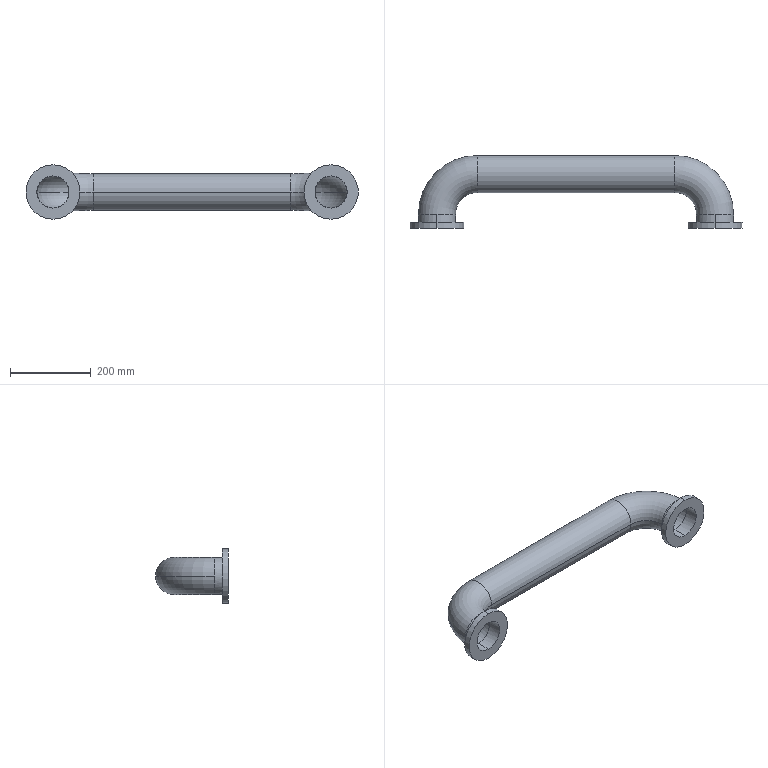Part | SolidWorks | features ICE 1, Sweep 1 | 1 solid | 28 faces | box 825 x 181 x 135 mm | volume 1647054 mm3 | cylinder 16 | torus 8 | plane 4 | commonest cylinder face diameters 80 x6 92 x6 135 x4
STEP:
#1=CARTESIAN_POINT('',(590.,80.,0.));
#2=VERTEX_POINT('',#1);
#3=CARTESIAN_POINT('',(590.,160.,0.));
#4=VERTEX_POINT('',#3);
#5=CARTESIAN_POINT('',(590.,120.,0.));
#6=DIRECTION('',(-1.,0.,0.));
#7=DIRECTION('',(0.,0.,1.));
#8=AXIS2_PLACEMENT_3D('',#5,#6,#7);
#9=CIRCLE('',#8,40.);
#10=EDGE_CURVE('',#2,#4,#9,.T.);
#11=ORIENTED_EDGE('',*,*,#10,.T.);
#12=CARTESIAN_POINT('',(730.,20.,0.));
#13=VERTEX_POINT('',#12);
#14=CARTESIAN_POINT('',(590.,20.,0.));
#15=DIRECTION('',(0.,0.,-1.));
#16=DIRECTION('',(-1.,0.,0.));
#17=AXIS2_PLACEMENT_3D('',#14,#15,#16);
#18=CIRCLE('',#17,140.);
#19=EDGE_CURVE('',#4,#13,#18,.T.);
#20=ORIENTED_EDGE('',*,*,#19,.T.);
#21=CARTESIAN_POINT('',(690.,20.,40.));
#22=VERTEX_POINT('',#21);
#23=CARTESIAN_POINT('',(690.,20.,0.));
#24=DIRECTION('',(0.,1.,0.));
#25=DIRECTION('',(0.,0.,1.));
#26=AXIS2_PLACEMENT_3D('',#23,#24,#25);
#27=CIRCLE('',#26,40.);
#28=EDGE_CURVE('',#22,#13,#27,.T.);
#29=ORIENTED_EDGE('',*,*,#28,.F.);
#30=CARTESIAN_POINT('',(650.,20.,0.));
#31=VERTEX_POINT('',#30);
#32=CARTESIAN_POINT('',(690.,20.,0.));
#33=DIRECTION('',(0.,1.,0.));
#34=DIRECTION('',(0.,0.,1.));
#35=AXIS2_PLACEMENT_3D('',#32,#33,#34);
#36=CIRCLE('',#35,40.);
#37=EDGE_CURVE('',#31,#22,#36,.T.);
#38=ORIENTED_EDGE('',*,*,#37,.F.);
#39=CARTESIAN_POINT('',(590.,20.,0.));
#40=DIRECTION('',(0.,0.,-1.));
#41=DIRECTION('',(-1.,0.,0.));
#42=AXIS2_PLACEMENT_3D('',#39,#40,#41);
#43=CIRCLE('',#42,60.);
#44=EDGE_CURVE('',#2,#31,#43,.T.);
#45=ORIENTED_EDGE('',*,*,#44,.F.);
#46=EDGE_LOOP('',(#11,#20,#29,#38,#45));
#47=FACE_OUTER_BOUND('',#46,.T.);
#48=CARTESIAN_POINT('',(590.,20.,0.));
#49=DIRECTION('',(0.,0.,-1.));
#50=DIRECTION('',(-1.,0.,0.));
#51=AXIS2_PLACEMENT_3D('',#48,#49,#50);
#52=TOROIDAL_SURFACE('',#51,100.,40.);
#53=ADVANCED_FACE('',(#47),#52,.F.);
#54=CARTESIAN_POINT('',(0.,20.,40.));
#55=VERTEX_POINT('',#54);
#56=CARTESIAN_POINT('',(-40.,20.,0.));
#57=VERTEX_POINT('',#56);
#58=CARTESIAN_POINT('',(0.,20.,0.));
#59=DIRECTION('',(0.,-1.,0.));
#60=DIRECTION('',(0.,0.,1.));
#61=AXIS2_PLACEMENT_3D('',#58,#59,#60);
#62=CIRCLE('',#61,40.);
#63=EDGE_CURVE('',#55,#57,#62,.T.);
#64=ORIENTED_EDGE('',*,*,#63,.T.);
#65=CARTESIAN_POINT('',(100.,160.,0.));
#66=VERTEX_POINT('',#65);
#67=CARTESIAN_POINT('',(100.,20.,0.));
#68=DIRECTION('',(0.,0.,-1.));
#69=DIRECTION('',(-1.,0.,0.));
#70=AXIS2_PLACEMENT_3D('',#67,#68,#69);
#71=CIRCLE('',#70,140.);
#72=EDGE_CURVE('',#57,#66,#71,.T.);
#73=ORIENTED_EDGE('',*,*,#72,.T.);
#74=CARTESIAN_POINT('',(100.,80.,0.));
#75=VERTEX_POINT('',#74);
#76=CARTESIAN_POINT('',(100.,120.,0.));
#77=DIRECTION('',(-1.,0.,0.));
#78=DIRECTION('',(0.,0.,1.));
#79=AXIS2_PLACEMENT_3D('',#76,#77,#78);
#80=CIRCLE('',#79,40.);
#81=EDGE_CURVE('',#75,#66,#80,.T.);
#82=ORIENTED_EDGE('',*,*,#81,.F.);
#83=CARTESIAN_POINT('',(40.,20.,0.));
#84=VERTEX_POINT('',#83);
#85=CARTESIAN_POINT('',(100.,20.,0.));
#86=DIRECTION('',(0.,0.,-1.));
#87=DIRECTION('',(-1.,0.,0.));
#88=AXIS2_PLACEMENT_3D('',#85,#86,#87);
#89=CIRCLE('',#88,60.);
#90=EDGE_CURVE('',#84,#75,#89,.T.);
#91=ORIENTED_EDGE('',*,*,#90,.F.);
#92=CARTESIAN_POINT('',(0.,20.,0.));
#93=DIRECTION('',(0.,-1.,0.));
#94=DIRECTION('',(0.,0.,1.));
#95=AXIS2_PLACEMENT_3D('',#92,#93,#94);
#96=CIRCLE('',#95,40.);
#97=EDGE_CURVE('',#84,#55,#96,.T.);
#98=ORIENTED_EDGE('',*,*,#97,.T.);
#99=EDGE_LOOP('',(#64,#73,#82,#91,#98));
#100=FACE_OUTER_BOUND('',#99,.T.);
#101=CARTESIAN_POINT('',(100.,20.,0.));
#102=DIRECTION('',(0.,0.,-1.));
#103=DIRECTION('',(-1.,0.,0.));
#104=AXIS2_PLACEMENT_3D('',#101,#102,#103);
#105=TOROIDAL_SURFACE('',#104,100.,40.);
#106=ADVANCED_FACE('',(#100),#105,.F.);
#107=CARTESIAN_POINT('',(590.,74.,0.));
#108=VERTEX_POINT('',#107);
#109=CARTESIAN_POINT('',(590.,166.,0.));
#110=VERTEX_POINT('',#109);
#111=CARTESIAN_POINT('',(590.,120.,0.));
#112=DIRECTION('',(1.,0.,0.));
#113=DIRECTION('',(0.,0.,1.));
#114=AXIS2_PLACEMENT_3D('',#111,#112,#113);
#115=CIRCLE('',#114,46.);
#116=EDGE_CURVE('',#108,#110,#115,.T.);
#117=ORIENTED_EDGE('',*,*,#116,.T.);
#118=CARTESIAN_POINT('',(736.,20.,0.));
#119=VERTEX_POINT('',#118);
#120=CARTESIAN_POINT('',(590.,20.,0.));
#121=DIRECTION('',(0.,0.,-1.));
#122=DIRECTION('',(-1.,0.,0.));
#123=AXIS2_PLACEMENT_3D('',#120,#121,#122);
#124=CIRCLE('',#123,146.);
#125=EDGE_CURVE('',#110,#119,#124,.T.);
#126=ORIENTED_EDGE('',*,*,#125,.T.);
#127=CARTESIAN_POINT('',(690.,20.,-46.));
#128=VERTEX_POINT('',#127);
#129=CARTESIAN_POINT('',(690.,20.,0.));
#130=DIRECTION('',(0.,-1.,0.));
#131=DIRECTION('',(0.,0.,1.));
#132=AXIS2_PLACEMENT_3D('',#129,#130,#131);
#133=CIRCLE('',#132,46.);
#134=EDGE_CURVE('',#128,#119,#133,.T.);
#135=ORIENTED_EDGE('',*,*,#134,.F.);
#136=CARTESIAN_POINT('',(644.,20.,0.));
#137=VERTEX_POINT('',#136);
#138=CARTESIAN_POINT('',(690.,20.,0.));
#139=DIRECTION('',(0.,-1.,0.));
#140=DIRECTION('',(0.,0.,1.));
#141=AXIS2_PLACEMENT_3D('',#138,#139,#140);
#142=CIRCLE('',#141,46.);
#143=EDGE_CURVE('',#137,#128,#142,.T.);
#144=ORIENTED_EDGE('',*,*,#143,.F.);
#145=CARTESIAN_POINT('',(590.,20.,0.));
#146=DIRECTION('',(0.,0.,-1.));
#147=DIRECTION('',(-1.,0.,0.));
#148=AXIS2_PLACEMENT_3D('',#145,#146,#147);
#149=CIRCLE('',#148,54.);
#150=EDGE_CURVE('',#108,#137,#149,.T.);
#151=ORIENTED_EDGE('',*,*,#150,.F.);
#152=EDGE_LOOP('',(#117,#126,#135,#144,#151));
#153=FACE_OUTER_BOUND('',#152,.T.);
#154=CARTESIAN_POINT('',(590.,20.,0.));
#155=DIRECTION('',(0.,0.,-1.));
#156=DIRECTION('',(-1.,0.,0.));
#157=AXIS2_PLACEMENT_3D('',#154,#155,#156);
#158=TOROIDAL_SURFACE('',#157,100.,46.);
#159=ADVANCED_FACE('',(#153),#158,.T.);
#160=CARTESIAN_POINT('',(0.,20.,-46.));
#161=VERTEX_POINT('',#160);
#162=CARTESIAN_POINT('',(-46.,20.,0.));
#163=VERTEX_POINT('',#162);
#164=CARTESIAN_POINT('',(0.,20.,0.));
#165=DIRECTION('',(0.,1.,0.));
#166=DIRECTION('',(0.,0.,1.));
#167=AXIS2_PLACEMENT_3D('',#164,#165,#166);
#168=CIRCLE('',#167,46.);
#169=EDGE_CURVE('',#161,#163,#168,.T.);
#170=ORIENTED_EDGE('',*,*,#169,.T.);
#171=CARTESIAN_POINT('',(100.,166.,0.));
#172=VERTEX_POINT('',#171);
#173=CARTESIAN_POINT('',(100.,20.,0.));
#174=DIRECTION('',(0.,0.,-1.));
#175=DIRECTION('',(-1.,0.,0.));
#176=AXIS2_PLACEMENT_3D('',#173,#174,#175);
#177=CIRCLE('',#176,146.);
#178=EDGE_CURVE('',#163,#172,#177,.T.);
#179=ORIENTED_EDGE('',*,*,#178,.T.);
#180=CARTESIAN_POINT('',(100.,74.,0.));
#181=VERTEX_POINT('',#180);
#182=CARTESIAN_POINT('',(100.,120.,0.));
#183=DIRECTION('',(1.,0.,0.));
#184=DIRECTION('',(0.,0.,1.));
#185=AXIS2_PLACEMENT_3D('',#182,#183,#184);
#186=CIRCLE('',#185,46.);
#187=EDGE_CURVE('',#181,#172,#186,.T.);
#188=ORIENTED_EDGE('',*,*,#187,.F.);
#189=CARTESIAN_POINT('',(46.,20.,0.));
#190=VERTEX_POINT('',#189);
#191=CARTESIAN_POINT('',(100.,20.,0.));
#192=DIRECTION('',(0.,0.,-1.));
#193=DIRECTION('',(-1.,0.,0.));
#194=AXIS2_PLACEMENT_3D('',#191,#192,#193);
#195=CIRCLE('',#194,54.);
#196=EDGE_CURVE('',#190,#181,#195,.T.);
#197=ORIENTED_EDGE('',*,*,#196,.F.);
#198=CARTESIAN_POINT('',(0.,20.,0.));
#199=DIRECTION('',(0.,1.,0.));
#200=DIRECTION('',(0.,0.,1.));
#201=AXIS2_PLACEMENT_3D('',#198,#199,#200);
#202=CIRCLE('',#201,46.);
#203=EDGE_CURVE('',#190,#161,#202,.T.);
#204=ORIENTED_EDGE('',*,*,#203,.T.);
#205=EDGE_LOOP('',(#170,#179,#188,#197,#204));
#206=FACE_OUTER_BOUND('',#205,.T.);
#207=CARTESIAN_POINT('',(100.,20.,0.));
#208=DIRECTION('',(0.,0.,-1.));
#209=DIRECTION('',(-1.,0.,0.));
#210=AXIS2_PLACEMENT_3D('',#207,#208,#209);
#211=TOROIDAL_SURFACE('',#210,100.,46.);
#212=ADVANCED_FACE('',(#206),#211,.T.);
#213=CARTESIAN_POINT('',(690.,-15.,-67.5));
#214=VERTEX_POINT('',#213);
#215=CARTESIAN_POINT('',(690.,-15.,67.5));
#216=VERTEX_POINT('',#215);
#217=CARTESIAN_POINT('',(690.,-15.,0.));
#218=DIRECTION('',(0.,-1.,0.));
#219=DIRECTION('',(0.,0.,-1.));
#220=AXIS2_PLACEMENT_3D('',#217,#218,#219);
#221=CIRCLE('',#220,67.5);
#222=EDGE_CURVE('',#214,#216,#221,.T.);
#223=ORIENTED_EDGE('',*,*,#222,.F.);
#224=CARTESIAN_POINT('',(690.,0.,-67.5));
#225=VERTEX_POINT('',#224);
#226=CARTESIAN_POINT('',(690.,-15.,-67.5));
#227=DIRECTION('',(0.,1.,0.));
#228=VECTOR('',#227,1000.);
#229=LINE('',#226,#228);
#230=EDGE_CURVE('',#214,#225,#229,.T.);
#231=ORIENTED_EDGE('',*,*,#230,.T.);
#232=CARTESIAN_POINT('',(690.,0.,67.5));
#233=VERTEX_POINT('',#232);
#234=CARTESIAN_POINT('',(690.,0.,0.));
#235=DIRECTION('',(0.,-1.,0.));
#236=DIRECTION('',(0.,0.,-1.));
#237=AXIS2_PLACEMENT_3D('',#234,#235,#236);
#238=CIRCLE('',#237,67.5);
#239=EDGE_CURVE('',#225,#233,#238,.T.);
#240=ORIENTED_EDGE('',*,*,#239,.T.);
#241=CARTESIAN_POINT('',(690.,-15.,67.5));
#242=DIRECTION('',(0.,1.,0.));
#243=VECTOR('',#242,1000.);
#244=LINE('',#241,#243);
#245=EDGE_CURVE('',#216,#233,#244,.T.);
#246=ORIENTED_EDGE('',*,*,#245,.F.);
#247=EDGE_LOOP('',(#223,#231,#240,#246));
#248=FACE_OUTER_BOUND('',#247,.T.);
#249=CARTESIAN_POINT('',(690.,-15.,0.));
#250=DIRECTION('',(0.,1.,0.));
#251=DIRECTION('',(0.,0.,1.));
#252=AXIS2_PLACEMENT_3D('',#249,#250,#251);
#253=CYLINDRICAL_SURFACE('',#252,67.5);
#254=ADVANCED_FACE('',(#248),#253,.T.);
#255=CARTESIAN_POINT('',(0.,-15.,-67.5));
#256=VERTEX_POINT('',#255);
#257=CARTESIAN_POINT('',(0.,-15.,67.5));
#258=VERTEX_POINT('',#257);
#259=CARTESIAN_POINT('',(0.,-15.,0.));
#260=DIRECTION('',(0.,-1.,0.));
#261=DIRECTION('',(0.,0.,-1.));
#262=AXIS2_PLACEMENT_3D('',#259,#260,#261);
#263=CIRCLE('',#262,67.5);
#264=EDGE_CURVE('',#256,#258,#263,.T.);
#265=ORIENTED_EDGE('',*,*,#264,.F.);
#266=CARTESIAN_POINT('',(0.,0.,-67.5));
#267=VERTEX_POINT('',#266);
#268=CARTESIAN_POINT('',(0.,-15.,-67.5));
#269=DIRECTION('',(0.,1.,0.));
#270=VECTOR('',#269,1000.);
#271=LINE('',#268,#270);
#272=EDGE_CURVE('',#256,#267,#271,.T.);
#273=ORIENTED_EDGE('',*,*,#272,.T.);
#274=CARTESIAN_POINT('',(0.,0.,67.5));
#275=VERTEX_POINT('',#274);
#276=CARTESIAN_POINT('',(0.,0.,0.));
#277=DIRECTION('',(0.,-1.,0.));
#278=DIRECTION('',(0.,0.,-1.));
#279=AXIS2_PLACEMENT_3D('',#276,#277,#278);
#280=CIRCLE('',#279,67.5);
#281=EDGE_CURVE('',#267,#275,#280,.T.);
#282=ORIENTED_EDGE('',*,*,#281,.T.);
#283=CARTESIAN_POINT('',(0.,-15.,67.5));
#284=DIRECTION('',(0.,1.,0.));
#285=VECTOR('',#284,1000.);
#286=LINE('',#283,#285);
#287=EDGE_CURVE('',#258,#275,#286,.T.);
#288=ORIENTED_EDGE('',*,*,#287,.F.);
#289=EDGE_LOOP('',(#265,#273,#282,#288));
#290=FACE_OUTER_BOUND('',#289,.T.);
#291=CARTESIAN_POINT('',(0.,-15.,0.));
#292=DIRECTION('',(0.,1.,0.));
#293=DIRECTION('',(0.,0.,1.));
#294=AXIS2_PLACEMENT_3D('',#291,#292,#293);
#295=CYLINDRICAL_SURFACE('',#294,67.5);
#296=ADVANCED_FACE('',(#290),#295,.T.);
#297=CARTESIAN_POINT('',(690.,20.,-40.));
#298=VERTEX_POINT('',#297);
#299=CARTESIAN_POINT('',(690.,20.,0.));
#300=DIRECTION('',(0.,1.,0.));
#301=DIRECTION('',(0.,0.,1.));
#302=AXIS2_PLACEMENT_3D('',#299,#300,#301);
#303=CIRCLE('',#302,40.);
#304=EDGE_CURVE('',#298,#31,#303,.T.);
#305=ORIENTED_EDGE('',*,*,#304,.T.);
#306=ORIENTED_EDGE('',*,*,#37,.T.);
#307=CARTESIAN_POINT('',(690.,-15.,40.));
#308=VERTEX_POINT('',#307);
#309=CARTESIAN_POINT('',(690.,20.,40.));
#310=DIRECTION('',(0.,-1.,0.));
#311=VECTOR('',#310,1000.);
#312=LINE('',#309,#311);
#313=EDGE_CURVE('',#22,#308,#312,.T.);
#314=ORIENTED_EDGE('',*,*,#313,.T.);
#315=CARTESIAN_POINT('',(690.,-15.,-40.));
#316=VERTEX_POINT('',#315);
#317=CARTESIAN_POINT('',(690.,-15.,0.));
#318=DIRECTION('',(0.,-1.,0.));
#319=DIRECTION('',(0.,0.,-1.));
#320=AXIS2_PLACEMENT_3D('',#317,#318,#319);
#321=CIRCLE('',#320,40.);
#322=EDGE_CURVE('',#308,#316,#321,.T.);
#323=ORIENTED_EDGE('',*,*,#322,.T.);
#324=CARTESIAN_POINT('',(690.,20.,-40.));
#325=DIRECTION('',(0.,-1.,0.));
#326=VECTOR('',#325,1000.);
#327=LINE('',#324,#326);
#328=EDGE_CURVE('',#298,#316,#327,.T.);
#329=ORIENTED_EDGE('',*,*,#328,.F.);
#330=EDGE_LOOP('',(#305,#306,#314,#323,#329));
#331=FACE_OUTER_BOUND('',#330,.T.);
#332=CARTESIAN_POINT('',(690.,20.,0.));
#333=DIRECTION('',(0.,-1.,0.));
#334=DIRECTION('',(0.,0.,-1.));
#335=AXIS2_PLACEMENT_3D('',#332,#333,#334);
#336=CYLINDRICAL_SURFACE('',#335,40.);
#337=ADVANCED_FACE('',(#331),#336,.F.);
#338=CARTESIAN_POINT('',(100.,120.,0.));
#339=DIRECTION('',(-1.,0.,0.));
#340=DIRECTION('',(0.,0.,1.));
#341=AXIS2_PLACEMENT_3D('',#338,#339,#340);
#342=CIRCLE('',#341,40.);
#343=EDGE_CURVE('',#66,#75,#342,.T.);
#344=ORIENTED_EDGE('',*,*,#343,.T.);
#345=CARTESIAN_POINT('',(100.,80.,0.));
#346=DIRECTION('',(1.,0.,0.));
#347=VECTOR('',#346,1000.);
#348=LINE('',#345,#347);
#349=EDGE_CURVE('',#75,#2,#348,.T.);
#350=ORIENTED_EDGE('',*,*,#349,.T.);
#351=CARTESIAN_POINT('',(590.,120.,0.));
#352=DIRECTION('',(-1.,0.,0.));
#353=DIRECTION('',(0.,0.,1.));
#354=AXIS2_PLACEMENT_3D('',#351,#352,#353);
#355=CIRCLE('',#354,40.);
#356=EDGE_CURVE('',#4,#2,#355,.T.);
#357=ORIENTED_EDGE('',*,*,#356,.F.);
#358=CARTESIAN_POINT('',(100.,160.,0.));
#359=DIRECTION('',(1.,0.,0.));
#360=VECTOR('',#359,1000.);
#361=LINE('',#358,#360);
#362=EDGE_CURVE('',#66,#4,#361,.T.);
#363=ORIENTED_EDGE('',*,*,#362,.F.);
#364=EDGE_LOOP('',(#344,#350,#357,#363));
#365=FACE_OUTER_BOUND('',#364,.T.);
#366=CARTESIAN_POINT('',(100.,120.,0.));
#367=DIRECTION('',(1.,0.,0.));
#368=DIRECTION('',(0.,1.,0.));
#369=AXIS2_PLACEMENT_3D('',#366,#367,#368);
#370=CYLINDRICAL_SURFACE('',#369,40.);
#371=ADVANCED_FACE('',(#365),#370,.F.);
#372=CARTESIAN_POINT('',(0.,-15.,40.));
#373=VERTEX_POINT('',#372);
#374=CARTESIAN_POINT('',(0.,-15.,-40.));
#375=VERTEX_POINT('',#374);
#376=CARTESIAN_POINT('',(0.,-15.,0.));
#377=DIRECTION('',(0.,-1.,0.));
#378=DIRECTION('',(0.,0.,-1.));
#379=AXIS2_PLACEMENT_3D('',#376,#377,#378);
#380=CIRCLE('',#379,40.);
#381=EDGE_CURVE('',#373,#375,#380,.T.);
#382=ORIENTED_EDGE('',*,*,#381,.T.);
#383=CARTESIAN_POINT('',(0.,20.,-40.));
#384=VERTEX_POINT('',#383);
#385=CARTESIAN_POINT('',(0.,0.,-40.));
#386=DIRECTION('',(0.,1.,0.));
#387=VECTOR('',#386,1000.);
#388=LINE('',#385,#387);
#389=EDGE_CURVE('',#375,#384,#388,.T.);
#390=ORIENTED_EDGE('',*,*,#389,.T.);
#391=CARTESIAN_POINT('',(0.,20.,0.));
#392=DIRECTION('',(0.,-1.,0.));
#393=DIRECTION('',(0.,0.,1.));
#394=AXIS2_PLACEMENT_3D('',#391,#392,#393);
#395=CIRCLE('',#394,40.);
#396=EDGE_CURVE('',#57,#384,#395,.T.);
#397=ORIENTED_EDGE('',*,*,#396,.F.);
#398=ORIENTED_EDGE('',*,*,#63,.F.);
#399=CARTESIAN_POINT('',(0.,0.,40.));
#400=DIRECTION('',(0.,1.,0.));
#401=VECTOR('',#400,1000.);
#402=LINE('',#399,#401);
#403=EDGE_CURVE('',#373,#55,#402,.T.);
#404=ORIENTED_EDGE('',*,*,#403,.F.);
#405=EDGE_LOOP('',(#382,#390,#397,#398,#404));
#406=FACE_OUTER_BOUND('',#405,.T.);
#407=CARTESIAN_POINT('',(0.,0.,0.));
#408=DIRECTION('',(0.,1.,0.));
#409=DIRECTION('',(0.,0.,1.));
#410=AXIS2_PLACEMENT_3D('',#407,#408,#409);
#411=CYLINDRICAL_SURFACE('',#410,40.);
#412=ADVANCED_FACE('',(#406),#411,.F.);
#413=ORIENTED_EDGE('',*,*,#134,.T.);
#414=CARTESIAN_POINT('',(690.,20.,46.));
#415=VERTEX_POINT('',#414);
#416=CARTESIAN_POINT('',(690.,20.,0.));
#417=DIRECTION('',(0.,-1.,0.));
#418=DIRECTION('',(0.,0.,1.));
#419=AXIS2_PLACEMENT_3D('',#416,#417,#418);
#420=CIRCLE('',#419,46.);
#421=EDGE_CURVE('',#119,#415,#420,.T.);
#422=ORIENTED_EDGE('',*,*,#421,.T.);
#423=CARTESIAN_POINT('',(690.,0.,46.));
#424=VERTEX_POINT('',#423);
#425=CARTESIAN_POINT('',(690.,20.,46.));
#426=DIRECTION('',(0.,-1.,0.));
#427=VECTOR('',#426,1000.);
#428=LINE('',#425,#427);
#429=EDGE_CURVE('',#415,#424,#428,.T.);
#430=ORIENTED_EDGE('',*,*,#429,.T.);
#431=CARTESIAN_POINT('',(690.,0.,-46.));
#432=VERTEX_POINT('',#431);
#433=CARTESIAN_POINT('',(690.,0.,0.));
#434=DIRECTION('',(0.,-1.,0.));
#435=DIRECTION('',(0.,0.,1.));
#436=AXIS2_PLACEMENT_3D('',#433,#434,#435);
#437=CIRCLE('',#436,46.);
#438=EDGE_CURVE('',#432,#424,#437,.T.);
#439=ORIENTED_EDGE('',*,*,#438,.F.);
#440=CARTESIAN_POINT('',(690.,20.,-46.));
#441=DIRECTION('',(0.,-1.,0.));
#442=VECTOR('',#441,1000.);
#443=LINE('',#440,#442);
#444=EDGE_CURVE('',#128,#432,#443,.T.);
#445=ORIENTED_EDGE('',*,*,#444,.F.);
#446=EDGE_LOOP('',(#413,#422,#430,#439,#445));
#447=FACE_OUTER_BOUND('',#446,.T.);
#448=CARTESIAN_POINT('',(690.,20.,0.));
#449=DIRECTION('',(0.,-1.,0.));
#450=DIRECTION('',(0.,0.,-1.));
#451=AXIS2_PLACEMENT_3D('',#448,#449,#450);
#452=CYLINDRICAL_SURFACE('',#451,46.);
#453=ADVANCED_FACE('',(#447),#452,.T.);
#454=CARTESIAN_POINT('',(100.,120.,0.));
#455=DIRECTION('',(1.,0.,0.));
#456=DIRECTION('',(0.,0.,1.));
#457=AXIS2_PLACEMENT_3D('',#454,#455,#456);
#458=CIRCLE('',#457,46.);
#459=EDGE_CURVE('',#172,#181,#458,.T.);
#460=ORIENTED_EDGE('',*,*,#459,.T.);
#461=CARTESIAN_POINT('',(100.,74.,0.));
#462=DIRECTION('',(1.,0.,0.));
#463=VECTOR('',#462,1000.);
#464=LINE('',#461,#463);
#465=EDGE_CURVE('',#181,#108,#464,.T.);
#466=ORIENTED_EDGE('',*,*,#465,.T.);
#467=CARTESIAN_POINT('',(590.,120.,0.));
#468=DIRECTION('',(1.,0.,0.));
#469=DIRECTION('',(0.,0.,1.));
#470=AXIS2_PLACEMENT_3D('',#467,#468,#469);
#471=CIRCLE('',#470,46.);
#472=EDGE_CURVE('',#110,#108,#471,.T.);
#473=ORIENTED_EDGE('',*,*,#472,.F.);
#474=CARTESIAN_POINT('',(100.,166.,0.));
#475=DIRECTION('',(1.,0.,0.));
#476=VECTOR('',#475,1000.);
#477=LINE('',#474,#476);
#478=EDGE_CURVE('',#172,#110,#477,.T.);
#479=ORIENTED_EDGE('',*,*,#478,.F.);
#480=EDGE_LOOP('',(#460,#466,#473,#479));
#481=FACE_OUTER_BOUND('',#480,.T.);
#482=CARTESIAN_POINT('',(100.,120.,0.));
#483=DIRECTION('',(1.,0.,0.));
#484=DIRECTION('',(0.,1.,0.));
#485=AXIS2_PLACEMENT_3D('',#482,#483,#484);
#486=CYLINDRICAL_SURFACE('',#485,46.);
#487=ADVANCED_FACE('',(#481),#486,.T.);
#488=CARTESIAN_POINT('',(0.,0.,46.));
#489=VERTEX_POINT('',#488);
#490=CARTESIAN_POINT('',(0.,0.,-46.));
#491=VERTEX_POINT('',#490);
#492=CARTESIAN_POINT('',(0.,0.,0.));
#493=DIRECTION('',(0.,1.,0.));
#494=DIRECTION('',(0.,0.,1.));
#495=AXIS2_PLACEMENT_3D('',#492,#493,#494);
#496=CIRCLE('',#495,46.);
#497=EDGE_CURVE('',#489,#491,#496,.T.);
#498=ORIENTED_EDGE('',*,*,#497,.T.);
#499=CARTESIAN_POINT('',(0.,0.,-46.));
#500=DIRECTION('',(0.,1.,0.));
#501=VECTOR('',#500,1000.);
#502=LINE('',#499,#501);
#503=EDGE_CURVE('',#491,#161,#502,.T.);
#504=ORIENTED_EDGE('',*,*,#503,.T.);
#505=ORIENTED_EDGE('',*,*,#203,.F.);
#506=CARTESIAN_POINT('',(0.,20.,46.));
#507=VERTEX_POINT('',#506);
#508=CARTESIAN_POINT('',(0.,20.,0.));
#509=DIRECTION('',(0.,1.,0.));
#510=DIRECTION('',(0.,0.,1.));
#511=AXIS2_PLACEMENT_3D('',#508,#509,#510);
#512=CIRCLE('',#511,46.);
#513=EDGE_CURVE('',#507,#190,#512,.T.);
#514=ORIENTED_EDGE('',*,*,#513,.F.);
#515=CARTESIAN_POINT('',(0.,0.,46.));
#516=DIRECTION('',(0.,1.,0.));
#517=VECTOR('',#516,1000.);
#518=LINE('',#515,#517);
#519=EDGE_CURVE('',#489,#507,#518,.T.);
#520=ORIENTED_EDGE('',*,*,#519,.F.);
#521=EDGE_LOOP('',(#498,#504,#505,#514,#520));
#522=FACE_OUTER_BOUND('',#521,.T.);
#523=CARTESIAN_POINT('',(0.,0.,0.));
#524=DIRECTION('',(0.,1.,0.));
#525=DIRECTION('',(0.,0.,1.));
#526=AXIS2_PLACEMENT_3D('',#523,#524,#525);
#527=CYLINDRICAL_SURFACE('',#526,46.);
#528=ADVANCED_FACE('',(#522),#527,.T.);
#529=ORIENTED_EDGE('',*,*,#313,.F.);
#530=ORIENTED_EDGE('',*,*,#28,.T.);
#531=CARTESIAN_POINT('',(690.,20.,0.));
#532=DIRECTION('',(0.,1.,0.));
#533=DIRECTION('',(0.,0.,1.));
#534=AXIS2_PLACEMENT_3D('',#531,#532,#533);
#535=CIRCLE('',#534,40.);
#536=EDGE_CURVE('',#13,#298,#535,.T.);
#537=ORIENTED_EDGE('',*,*,#536,.T.);
#538=ORIENTED_EDGE('',*,*,#328,.T.);
#539=CARTESIAN_POINT('',(690.,-15.,0.));
#540=DIRECTION('',(0.,-1.,0.));
#541=DIRECTION('',(0.,0.,-1.));
#542=AXIS2_PLACEMENT_3D('',#539,#540,#541);
#543=CIRCLE('',#542,40.);
#544=EDGE_CURVE('',#316,#308,#543,.T.);
#545=ORIENTED_EDGE('',*,*,#544,.T.);
#546=EDGE_LOOP('',(#529,#530,#537,#538,#545));
#547=FACE_OUTER_BOUND('',#546,.T.);
#548=CARTESIAN_POINT('',(690.,20.,0.));
#549=DIRECTION('',(0.,-1.,0.));
#550=DIRECTION('',(0.,0.,-1.));
#551=AXIS2_PLACEMENT_3D('',#548,#549,#550);
#552=CYLINDRICAL_SURFACE('',#551,40.);
#553=ADVANCED_FACE('',(#547),#552,.F.);
#554=ORIENTED_EDGE('',*,*,#19,.F.);
#555=ORIENTED_EDGE('',*,*,#356,.T.);
#556=ORIENTED_EDGE('',*,*,#44,.T.);
#557=ORIENTED_EDGE('',*,*,#304,.F.);
#558=ORIENTED_EDGE('',*,*,#536,.F.);
#559=EDGE_LOOP('',(#554,#555,#556,#557,#558));
#560=FACE_OUTER_BOUND('',#559,.T.);
#561=CARTESIAN_POINT('',(590.,20.,0.));
#562=DIRECTION('',(0.,0.,-1.));
#563=DIRECTION('',(-1.,0.,0.));
#564=AXIS2_PLACEMENT_3D('',#561,#562,#563);
#565=TOROIDAL_SURFACE('',#564,100.,40.);
#566=ADVANCED_FACE('',(#560),#565,.F.);
#567=ORIENTED_EDGE('',*,*,#349,.F.);
#568=ORIENTED_EDGE('',*,*,#81,.T.);
#569=ORIENTED_EDGE('',*,*,#362,.T.);
#570=ORIENTED_EDGE('',*,*,#10,.F.);
#571=EDGE_LOOP('',(#567,#568,#569,#570));
#572=FACE_OUTER_BOUND('',#571,.T.);
#573=CARTESIAN_POINT('',(100.,120.,0.));
#574=DIRECTION('',(1.,0.,0.));
#575=DIRECTION('',(0.,1.,0.));
#576=AXIS2_PLACEMENT_3D('',#573,#574,#575);
#577=CYLINDRICAL_SURFACE('',#576,40.);
#578=ADVANCED_FACE('',(#572),#577,.F.);
#579=ORIENTED_EDGE('',*,*,#72,.F.);
#580=ORIENTED_EDGE('',*,*,#396,.T.);
#581=CARTESIAN_POINT('',(0.,20.,0.));
#582=DIRECTION('',(0.,-1.,0.));
#583=DIRECTION('',(0.,0.,1.));
#584=AXIS2_PLACEMENT_3D('',#581,#582,#583);
#585=CIRCLE('',#584,40.);
#586=EDGE_CURVE('',#384,#84,#585,.T.);
#587=ORIENTED_EDGE('',*,*,#586,.T.);
#588=ORIENTED_EDGE('',*,*,#90,.T.);
#589=ORIENTED_EDGE('',*,*,#343,.F.);
#590=EDGE_LOOP('',(#579,#580,#587,#588,#589));
#591=FACE_OUTER_BOUND('',#590,.T.);
#592=CARTESIAN_POINT('',(100.,20.,0.));
#593=DIRECTION('',(0.,0.,-1.));
#594=DIRECTION('',(-1.,0.,0.));
#595=AXIS2_PLACEMENT_3D('',#592,#593,#594);
#596=TOROIDAL_SURFACE('',#595,100.,40.);
#597=ADVANCED_FACE('',(#591),#596,.F.);
#598=ORIENTED_EDGE('',*,*,#389,.F.);
#599=CARTESIAN_POINT('',(0.,-15.,0.));
#600=DIRECTION('',(0.,-1.,0.));
#601=DIRECTION('',(0.,0.,-1.));
#602=AXIS2_PLACEMENT_3D('',#599,#600,#601);
#603=CIRCLE('',#602,40.);
#604=EDGE_CURVE('',#375,#373,#603,.T.);
#605=ORIENTED_EDGE('',*,*,#604,.T.);
#606=ORIENTED_EDGE('',*,*,#403,.T.);
#607=ORIENTED_EDGE('',*,*,#97,.F.);
#608=ORIENTED_EDGE('',*,*,#586,.F.);
#609=EDGE_LOOP('',(#598,#605,#606,#607,#608));
#610=FACE_OUTER_BOUND('',#609,.T.);
#611=CARTESIAN_POINT('',(0.,0.,0.));
#612=DIRECTION('',(0.,1.,0.));
#613=DIRECTION('',(0.,0.,1.));
#614=AXIS2_PLACEMENT_3D('',#611,#612,#613);
#615=CYLINDRICAL_SURFACE('',#614,40.);
#616=ADVANCED_FACE('',(#610),#615,.F.);
#617=ORIENTED_EDGE('',*,*,#429,.F.);
#618=CARTESIAN_POINT('',(690.,20.,0.));
#619=DIRECTION('',(0.,-1.,0.));
#620=DIRECTION('',(0.,0.,1.));
#621=AXIS2_PLACEMENT_3D('',#618,#619,#620);
#622=CIRCLE('',#621,46.);
#623=EDGE_CURVE('',#415,#137,#622,.T.);
#624=ORIENTED_EDGE('',*,*,#623,.T.);
#625=ORIENTED_EDGE('',*,*,#143,.T.);
#626=ORIENTED_EDGE('',*,*,#444,.T.);
#627=CARTESIAN_POINT('',(690.,0.,0.));
#628=DIRECTION('',(0.,-1.,0.));
#629=DIRECTION('',(0.,0.,1.));
#630=AXIS2_PLACEMENT_3D('',#627,#628,#629);
#631=CIRCLE('',#630,46.);
#632=EDGE_CURVE('',#424,#432,#631,.T.);
#633=ORIENTED_EDGE('',*,*,#632,.F.);
#634=EDGE_LOOP('',(#617,#624,#625,#626,#633));
#635=FACE_OUTER_BOUND('',#634,.T.);
#636=CARTESIAN_POINT('',(690.,20.,0.));
#637=DIRECTION('',(0.,-1.,0.));
#638=DIRECTION('',(0.,0.,-1.));
#639=AXIS2_PLACEMENT_3D('',#636,#637,#638);
#640=CYLINDRICAL_SURFACE('',#639,46.);
#641=ADVANCED_FACE('',(#635),#640,.T.);
#642=ORIENTED_EDGE('',*,*,#125,.F.);
#643=ORIENTED_EDGE('',*,*,#472,.T.);
#644=ORIENTED_EDGE('',*,*,#150,.T.);
#645=ORIENTED_EDGE('',*,*,#623,.F.);
#646=ORIENTED_EDGE('',*,*,#421,.F.);
#647=EDGE_LOOP('',(#642,#643,#644,#645,#646));
#648=FACE_OUTER_BOUND('',#647,.T.);
#649=CARTESIAN_POINT('',(590.,20.,0.));
#650=DIRECTION('',(0.,0.,-1.));
#651=DIRECTION('',(-1.,0.,0.));
#652=AXIS2_PLACEMENT_3D('',#649,#650,#651);
#653=TOROIDAL_SURFACE('',#652,100.,46.);
#654=ADVANCED_FACE('',(#648),#653,.T.);
#655=ORIENTED_EDGE('',*,*,#465,.F.);
#656=ORIENTED_EDGE('',*,*,#187,.T.);
#657=ORIENTED_EDGE('',*,*,#478,.T.);
#658=ORIENTED_EDGE('',*,*,#116,.F.);
#659=EDGE_LOOP('',(#655,#656,#657,#658));
#660=FACE_OUTER_BOUND('',#659,.T.);
#661=CARTESIAN_POINT('',(100.,120.,0.));
#662=DIRECTION('',(1.,0.,0.));
#663=DIRECTION('',(0.,1.,0.));
#664=AXIS2_PLACEMENT_3D('',#661,#662,#663);
#665=CYLINDRICAL_SURFACE('',#664,46.);
#666=ADVANCED_FACE('',(#660),#665,.T.);
#667=ORIENTED_EDGE('',*,*,#178,.F.);
#668=CARTESIAN_POINT('',(0.,20.,0.));
#669=DIRECTION('',(0.,1.,0.));
#670=DIRECTION('',(0.,0.,1.));
#671=AXIS2_PLACEMENT_3D('',#668,#669,#670);
#672=CIRCLE('',#671,46.);
#673=EDGE_CURVE('',#163,#507,#672,.T.);
#674=ORIENTED_EDGE('',*,*,#673,.T.);
#675=ORIENTED_EDGE('',*,*,#513,.T.);
#676=ORIENTED_EDGE('',*,*,#196,.T.);
#677=ORIENTED_EDGE('',*,*,#459,.F.);
#678=EDGE_LOOP('',(#667,#674,#675,#676,#677));
#679=FACE_OUTER_BOUND('',#678,.T.);
#680=CARTESIAN_POINT('',(100.,20.,0.));
#681=DIRECTION('',(0.,0.,-1.));
#682=DIRECTION('',(-1.,0.,0.));
#683=AXIS2_PLACEMENT_3D('',#680,#681,#682);
#684=TOROIDAL_SURFACE('',#683,100.,46.);
#685=ADVANCED_FACE('',(#679),#684,.T.);
#686=ORIENTED_EDGE('',*,*,#503,.F.);
#687=CARTESIAN_POINT('',(0.,0.,0.));
#688=DIRECTION('',(0.,1.,0.));
#689=DIRECTION('',(0.,0.,1.));
#690=AXIS2_PLACEMENT_3D('',#687,#688,#689);
#691=CIRCLE('',#690,46.);
#692=EDGE_CURVE('',#491,#489,#691,.T.);
#693=ORIENTED_EDGE('',*,*,#692,.T.);
#694=ORIENTED_EDGE('',*,*,#519,.T.);
#695=ORIENTED_EDGE('',*,*,#673,.F.);
#696=ORIENTED_EDGE('',*,*,#169,.F.);
#697=EDGE_LOOP('',(#686,#693,#694,#695,#696));
#698=FACE_OUTER_BOUND('',#697,.T.);
#699=CARTESIAN_POINT('',(0.,0.,0.));
#700=DIRECTION('',(0.,1.,0.));
#701=DIRECTION('',(0.,0.,1.));
#702=AXIS2_PLACEMENT_3D('',#699,#700,#701);
#703=CYLINDRICAL_SURFACE('',#702,46.);
#704=ADVANCED_FACE('',(#698),#703,.T.);
#705=CARTESIAN_POINT('',(0.,-15.,0.));
#706=DIRECTION('',(0.,-1.,0.));
#707=DIRECTION('',(0.,0.,-1.));
#708=AXIS2_PLACEMENT_3D('',#705,#706,#707);
#709=CIRCLE('',#708,67.5);
#710=EDGE_CURVE('',#258,#256,#709,.T.);
#711=ORIENTED_EDGE('',*,*,#710,.T.);
#712=ORIENTED_EDGE('',*,*,#264,.T.);
#713=EDGE_LOOP('',(#711,#712));
#714=FACE_OUTER_BOUND('',#713,.T.);
#715=ORIENTED_EDGE('',*,*,#381,.F.);
#716=ORIENTED_EDGE('',*,*,#604,.F.);
#717=EDGE_LOOP('',(#715,#716));
#718=FACE_BOUND('',#717,.T.);
#719=CARTESIAN_POINT('',(0.,-15.,0.));
#720=DIRECTION('',(0.,-1.,0.));
#721=DIRECTION('',(0.,0.,-1.));
#722=AXIS2_PLACEMENT_3D('',#719,#720,#721);
#723=PLANE('',#722);
#724=ADVANCED_FACE('',(#714,#718),#723,.T.);
#725=ORIENTED_EDGE('',*,*,#497,.F.);
#726=ORIENTED_EDGE('',*,*,#692,.F.);
#727=EDGE_LOOP('',(#725,#726));
#728=FACE_BOUND('',#727,.T.);
#729=CARTESIAN_POINT('',(0.,0.,0.));
#730=DIRECTION('',(0.,-1.,0.));
#731=DIRECTION('',(0.,0.,-1.));
#732=AXIS2_PLACEMENT_3D('',#729,#730,#731);
#733=CIRCLE('',#732,67.5);
#734=EDGE_CURVE('',#275,#267,#733,.T.);
#735=ORIENTED_EDGE('',*,*,#734,.F.);
#736=ORIENTED_EDGE('',*,*,#281,.F.);
#737=EDGE_LOOP('',(#735,#736));
#738=FACE_OUTER_BOUND('',#737,.T.);
#739=CARTESIAN_POINT('',(0.,0.,0.));
#740=DIRECTION('',(0.,-1.,0.));
#741=DIRECTION('',(0.,0.,-1.));
#742=AXIS2_PLACEMENT_3D('',#739,#740,#741);
#743=PLANE('',#742);
#744=ADVANCED_FACE('',(#728,#738),#743,.F.);
#745=ORIENTED_EDGE('',*,*,#272,.F.);
#746=ORIENTED_EDGE('',*,*,#710,.F.);
#747=ORIENTED_EDGE('',*,*,#287,.T.);
#748=ORIENTED_EDGE('',*,*,#734,.T.);
#749=EDGE_LOOP('',(#745,#746,#747,#748));
#750=FACE_OUTER_BOUND('',#749,.T.);
#751=CARTESIAN_POINT('',(0.,-15.,0.));
#752=DIRECTION('',(0.,1.,0.));
#753=DIRECTION('',(0.,0.,1.));
#754=AXIS2_PLACEMENT_3D('',#751,#752,#753);
#755=CYLINDRICAL_SURFACE('',#754,67.5);
#756=ADVANCED_FACE('',(#750),#755,.T.);
#757=CARTESIAN_POINT('',(690.,-15.,0.));
#758=DIRECTION('',(0.,-1.,0.));
#759=DIRECTION('',(0.,0.,-1.));
#760=AXIS2_PLACEMENT_3D('',#757,#758,#759);
#761=CIRCLE('',#760,67.5);
#762=EDGE_CURVE('',#216,#214,#761,.T.);
#763=ORIENTED_EDGE('',*,*,#762,.T.);
#764=ORIENTED_EDGE('',*,*,#222,.T.);
#765=EDGE_LOOP('',(#763,#764));
#766=FACE_OUTER_BOUND('',#765,.T.);
#767=ORIENTED_EDGE('',*,*,#544,.F.);
#768=ORIENTED_EDGE('',*,*,#322,.F.);
#769=EDGE_LOOP('',(#767,#768));
#770=FACE_BOUND('',#769,.T.);
#771=CARTESIAN_POINT('',(690.,-15.,0.));
#772=DIRECTION('',(0.,-1.,0.));
#773=DIRECTION('',(0.,0.,-1.));
#774=AXIS2_PLACEMENT_3D('',#771,#772,#773);
#775=PLANE('',#774);
#776=ADVANCED_FACE('',(#766,#770),#775,.T.);
#777=ORIENTED_EDGE('',*,*,#438,.T.);
#778=ORIENTED_EDGE('',*,*,#632,.T.);
#779=EDGE_LOOP('',(#777,#778));
#780=FACE_BOUND('',#779,.T.);
#781=CARTESIAN_POINT('',(690.,0.,0.));
#782=DIRECTION('',(0.,-1.,0.));
#783=DIRECTION('',(0.,0.,-1.));
#784=AXIS2_PLACEMENT_3D('',#781,#782,#783);
#785=CIRCLE('',#784,67.5);
#786=EDGE_CURVE('',#233,#225,#785,.T.);
#787=ORIENTED_EDGE('',*,*,#786,.F.);
#788=ORIENTED_EDGE('',*,*,#239,.F.);
#789=EDGE_LOOP('',(#787,#788));
#790=FACE_OUTER_BOUND('',#789,.T.);
#791=CARTESIAN_POINT('',(690.,0.,0.));
#792=DIRECTION('',(0.,-1.,0.));
#793=DIRECTION('',(0.,0.,-1.));
#794=AXIS2_PLACEMENT_3D('',#791,#792,#793);
#795=PLANE('',#794);
#796=ADVANCED_FACE('',(#780,#790),#795,.F.);
#797=ORIENTED_EDGE('',*,*,#230,.F.);
#798=ORIENTED_EDGE('',*,*,#762,.F.);
#799=ORIENTED_EDGE('',*,*,#245,.T.);
#800=ORIENTED_EDGE('',*,*,#786,.T.);
#801=EDGE_LOOP('',(#797,#798,#799,#800));
#802=FACE_OUTER_BOUND('',#801,.T.);
#803=CARTESIAN_POINT('',(690.,-15.,0.));
#804=DIRECTION('',(0.,1.,0.));
#805=DIRECTION('',(0.,0.,1.));
#806=AXIS2_PLACEMENT_3D('',#803,#804,#805);
#807=CYLINDRICAL_SURFACE('',#806,67.5);
#808=ADVANCED_FACE('',(#802),#807,.T.);
#809=CLOSED_SHELL('',(#53,#106,#159,#212,#254,#296,#337,#371,#412,#453,#487,#528,#553,#566,#578,#597,#616,#641,#654,#666,#685,#704,#724,#744,#756,#776,#796,#808));
#810=MANIFOLD_SOLID_BREP('',#809);
#811=CARTESIAN_POINT('',(0.,0.,0.));
#812=DIRECTION('',(0.,0.,1.));
#813=DIRECTION('',(1.,0.,0.));
#814=AXIS2_PLACEMENT_3D('',#811,#812,#813);
#815=(LENGTH_UNIT()NAMED_UNIT(*)SI_UNIT(.MILLI.,.METRE.));
#816=UNCERTAINTY_MEASURE_WITH_UNIT(LENGTH_MEASURE(0.00001),#815,'','');
#817=(NAMED_UNIT(*)PLANE_ANGLE_UNIT()SI_UNIT($,.RADIAN.));
#818=(NAMED_UNIT(*)SI_UNIT($,.STERADIAN.)SOLID_ANGLE_UNIT());
#819=(GEOMETRIC_REPRESENTATION_CONTEXT(3)GLOBAL_UNCERTAINTY_ASSIGNED_CONTEXT((#816))GLOBAL_UNIT_ASSIGNED_CONTEXT((#815,#817,#818))REPRESENTATION_CONTEXT('',''));
#820=ADVANCED_BREP_SHAPE_REPRESENTATION('',(#810,#814),#819);